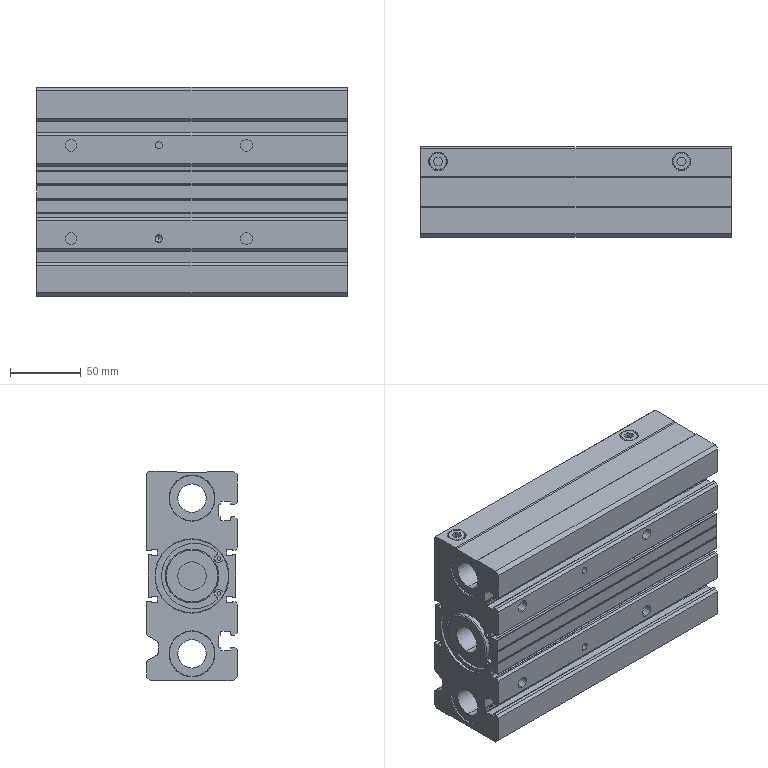Part | STEP file | TC_L_50x175175_b | 1 solid | 404 faces | box 219 x 64 x 148 mm | volume 1265791 mm3 | cylinder 184 | plane 154 | cone 62 | torus 4 | commonest cylinder face diameters 0.4 x32 0.8 x28 8.376 x16 3 x14 5 x14 20 x10